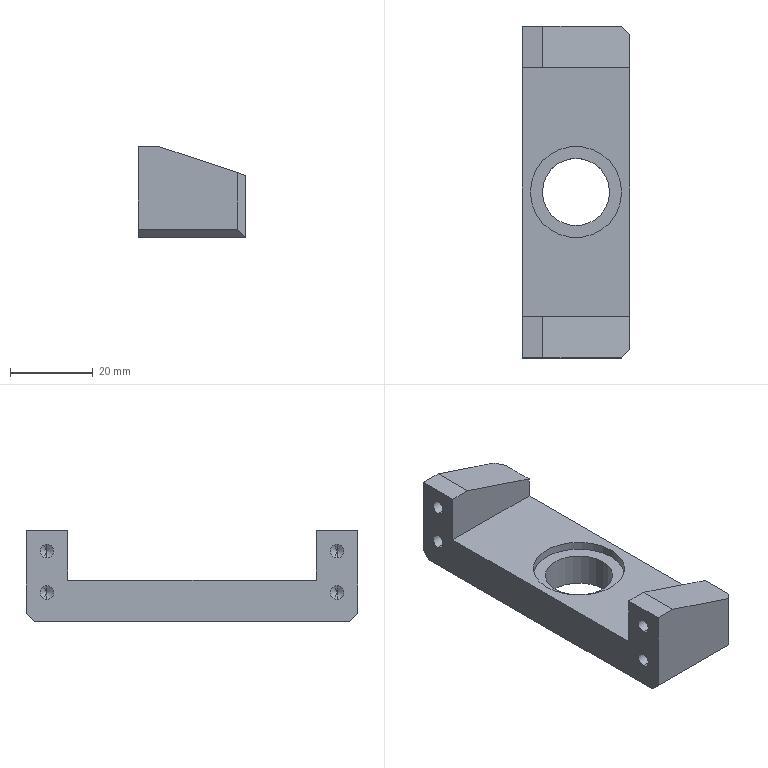Part | SolidWorks | features Chamfer 2, Cut 2, Extrusion 1, HoleWzd 1, ICE 1, MirrorPattern 1 | 1 solid | 37 faces | box 26 x 80 x 22 mm | volume 22644 mm3 | plane 17 | cylinder 12 | cone 8 | commonest cylinder face diameters 3.3 x8 16.2 x2 22 x2
STEP:
#1=CARTESIAN_POINT('',(-2.9,35.,15.35));
#2=VERTEX_POINT('',#1);
#3=CARTESIAN_POINT('',(-2.9,35.,18.65));
#4=VERTEX_POINT('',#3);
#5=CARTESIAN_POINT('',(-2.9,35.,17.));
#6=DIRECTION('',(-1.,0.,0.));
#7=DIRECTION('',(0.,0.,1.));
#8=AXIS2_PLACEMENT_3D('',#5,#6,#7);
#9=CIRCLE('',#8,1.65);
#10=EDGE_CURVE('',#2,#4,#9,.T.);
#11=ORIENTED_EDGE('',*,*,#10,.F.);
#12=CARTESIAN_POINT('',(-13.,35.,15.35));
#13=VERTEX_POINT('',#12);
#14=CARTESIAN_POINT('',(-13.,35.,15.35));
#15=DIRECTION('',(-1.,0.,0.));
#16=VECTOR('',#15,1000.);
#17=LINE('',#14,#16);
#18=EDGE_CURVE('',#2,#13,#17,.T.);
#19=ORIENTED_EDGE('',*,*,#18,.T.);
#20=CARTESIAN_POINT('',(-13.,35.,18.65));
#21=VERTEX_POINT('',#20);
#22=CARTESIAN_POINT('',(-13.,35.,17.));
#23=DIRECTION('',(-1.,0.,0.));
#24=DIRECTION('',(0.,0.,1.));
#25=AXIS2_PLACEMENT_3D('',#22,#23,#24);
#26=CIRCLE('',#25,1.65);
#27=EDGE_CURVE('',#13,#21,#26,.T.);
#28=ORIENTED_EDGE('',*,*,#27,.T.);
#29=CARTESIAN_POINT('',(-13.,35.,18.65));
#30=DIRECTION('',(-1.,0.,0.));
#31=VECTOR('',#30,1000.);
#32=LINE('',#29,#31);
#33=EDGE_CURVE('',#4,#21,#32,.T.);
#34=ORIENTED_EDGE('',*,*,#33,.F.);
#35=EDGE_LOOP('',(#11,#19,#28,#34));
#36=FACE_OUTER_BOUND('',#35,.T.);
#37=CARTESIAN_POINT('',(-13.,35.,17.));
#38=DIRECTION('',(-1.,0.,0.));
#39=DIRECTION('',(0.,0.,1.));
#40=AXIS2_PLACEMENT_3D('',#37,#38,#39);
#41=CYLINDRICAL_SURFACE('',#40,1.65);
#42=ADVANCED_FACE('',(#36),#41,.F.);
#43=CARTESIAN_POINT('',(-1.909,35.,17.));
#44=VERTEX_POINT('',#43);
#45=CARTESIAN_POINT('',(-2.9,35.,18.65));
#46=DIRECTION('',(-0.515,0.,0.8572));
#47=VECTOR('',#46,1000.);
#48=LINE('',#45,#47);
#49=EDGE_CURVE('',#44,#4,#48,.T.);
#50=ORIENTED_EDGE('',*,*,#49,.F.);
#51=CARTESIAN_POINT('',(-2.9,35.,15.35));
#52=DIRECTION('',(-0.515,0.,-0.8572));
#53=VECTOR('',#52,1000.);
#54=LINE('',#51,#53);
#55=EDGE_CURVE('',#44,#2,#54,.T.);
#56=ORIENTED_EDGE('',*,*,#55,.T.);
#57=ORIENTED_EDGE('',*,*,#10,.T.);
#58=EDGE_LOOP('',(#50,#56,#57));
#59=FACE_OUTER_BOUND('',#58,.T.);
#60=CARTESIAN_POINT('',(-2.9,35.,17.));
#61=DIRECTION('',(-1.,0.,0.));
#62=DIRECTION('',(0.,0.,1.));
#63=AXIS2_PLACEMENT_3D('',#60,#61,#62);
#64=CONICAL_SURFACE('',#63,1.65,1.03);
#65=ADVANCED_FACE('',(#59),#64,.F.);
#66=CARTESIAN_POINT('',(-2.9,35.,5.35));
#67=VERTEX_POINT('',#66);
#68=CARTESIAN_POINT('',(-2.9,35.,8.65));
#69=VERTEX_POINT('',#68);
#70=CARTESIAN_POINT('',(-2.9,35.,7.));
#71=DIRECTION('',(-1.,0.,0.));
#72=DIRECTION('',(0.,0.,1.));
#73=AXIS2_PLACEMENT_3D('',#70,#71,#72);
#74=CIRCLE('',#73,1.65);
#75=EDGE_CURVE('',#67,#69,#74,.T.);
#76=ORIENTED_EDGE('',*,*,#75,.F.);
#77=CARTESIAN_POINT('',(-13.,35.,5.35));
#78=VERTEX_POINT('',#77);
#79=CARTESIAN_POINT('',(-13.,35.,5.35));
#80=DIRECTION('',(-1.,0.,0.));
#81=VECTOR('',#80,1000.);
#82=LINE('',#79,#81);
#83=EDGE_CURVE('',#67,#78,#82,.T.);
#84=ORIENTED_EDGE('',*,*,#83,.T.);
#85=CARTESIAN_POINT('',(-13.,35.,8.65));
#86=VERTEX_POINT('',#85);
#87=CARTESIAN_POINT('',(-13.,35.,7.));
#88=DIRECTION('',(-1.,0.,0.));
#89=DIRECTION('',(0.,0.,1.));
#90=AXIS2_PLACEMENT_3D('',#87,#88,#89);
#91=CIRCLE('',#90,1.65);
#92=EDGE_CURVE('',#78,#86,#91,.T.);
#93=ORIENTED_EDGE('',*,*,#92,.T.);
#94=CARTESIAN_POINT('',(-13.,35.,8.65));
#95=DIRECTION('',(-1.,0.,0.));
#96=VECTOR('',#95,1000.);
#97=LINE('',#94,#96);
#98=EDGE_CURVE('',#69,#86,#97,.T.);
#99=ORIENTED_EDGE('',*,*,#98,.F.);
#100=EDGE_LOOP('',(#76,#84,#93,#99));
#101=FACE_OUTER_BOUND('',#100,.T.);
#102=CARTESIAN_POINT('',(-13.,35.,7.));
#103=DIRECTION('',(-1.,0.,0.));
#104=DIRECTION('',(0.,0.,1.));
#105=AXIS2_PLACEMENT_3D('',#102,#103,#104);
#106=CYLINDRICAL_SURFACE('',#105,1.65);
#107=ADVANCED_FACE('',(#101),#106,.F.);
#108=CARTESIAN_POINT('',(-1.909,35.,7.));
#109=VERTEX_POINT('',#108);
#110=CARTESIAN_POINT('',(-2.9,35.,8.65));
#111=DIRECTION('',(-0.515,0.,0.8572));
#112=VECTOR('',#111,1000.);
#113=LINE('',#110,#112);
#114=EDGE_CURVE('',#109,#69,#113,.T.);
#115=ORIENTED_EDGE('',*,*,#114,.F.);
#116=CARTESIAN_POINT('',(-2.9,35.,5.35));
#117=DIRECTION('',(-0.515,0.,-0.8572));
#118=VECTOR('',#117,1000.);
#119=LINE('',#116,#118);
#120=EDGE_CURVE('',#109,#67,#119,.T.);
#121=ORIENTED_EDGE('',*,*,#120,.T.);
#122=ORIENTED_EDGE('',*,*,#75,.T.);
#123=EDGE_LOOP('',(#115,#121,#122));
#124=FACE_OUTER_BOUND('',#123,.T.);
#125=CARTESIAN_POINT('',(-2.9,35.,7.));
#126=DIRECTION('',(-1.,0.,0.));
#127=DIRECTION('',(0.,0.,1.));
#128=AXIS2_PLACEMENT_3D('',#125,#126,#127);
#129=CONICAL_SURFACE('',#128,1.65,1.03);
#130=ADVANCED_FACE('',(#124),#129,.F.);
#131=CARTESIAN_POINT('',(-2.9,-35.,5.35));
#132=VERTEX_POINT('',#131);
#133=CARTESIAN_POINT('',(-2.9,-35.,8.65));
#134=VERTEX_POINT('',#133);
#135=CARTESIAN_POINT('',(-2.9,-35.,7.));
#136=DIRECTION('',(-1.,0.,0.));
#137=DIRECTION('',(0.,0.,1.));
#138=AXIS2_PLACEMENT_3D('',#135,#136,#137);
#139=CIRCLE('',#138,1.65);
#140=EDGE_CURVE('',#132,#134,#139,.T.);
#141=ORIENTED_EDGE('',*,*,#140,.F.);
#142=CARTESIAN_POINT('',(-13.,-35.,5.35));
#143=VERTEX_POINT('',#142);
#144=CARTESIAN_POINT('',(-13.,-35.,5.35));
#145=DIRECTION('',(-1.,0.,0.));
#146=VECTOR('',#145,1000.);
#147=LINE('',#144,#146);
#148=EDGE_CURVE('',#132,#143,#147,.T.);
#149=ORIENTED_EDGE('',*,*,#148,.T.);
#150=CARTESIAN_POINT('',(-13.,-35.,8.65));
#151=VERTEX_POINT('',#150);
#152=CARTESIAN_POINT('',(-13.,-35.,7.));
#153=DIRECTION('',(-1.,0.,0.));
#154=DIRECTION('',(0.,0.,1.));
#155=AXIS2_PLACEMENT_3D('',#152,#153,#154);
#156=CIRCLE('',#155,1.65);
#157=EDGE_CURVE('',#143,#151,#156,.T.);
#158=ORIENTED_EDGE('',*,*,#157,.T.);
#159=CARTESIAN_POINT('',(-13.,-35.,8.65));
#160=DIRECTION('',(-1.,0.,0.));
#161=VECTOR('',#160,1000.);
#162=LINE('',#159,#161);
#163=EDGE_CURVE('',#134,#151,#162,.T.);
#164=ORIENTED_EDGE('',*,*,#163,.F.);
#165=EDGE_LOOP('',(#141,#149,#158,#164));
#166=FACE_OUTER_BOUND('',#165,.T.);
#167=CARTESIAN_POINT('',(-13.,-35.,7.));
#168=DIRECTION('',(-1.,0.,0.));
#169=DIRECTION('',(0.,0.,1.));
#170=AXIS2_PLACEMENT_3D('',#167,#168,#169);
#171=CYLINDRICAL_SURFACE('',#170,1.65);
#172=ADVANCED_FACE('',(#166),#171,.F.);
#173=CARTESIAN_POINT('',(-1.909,-35.,7.));
#174=VERTEX_POINT('',#173);
#175=CARTESIAN_POINT('',(-2.9,-35.,8.65));
#176=DIRECTION('',(-0.515,0.,0.8572));
#177=VECTOR('',#176,1000.);
#178=LINE('',#175,#177);
#179=EDGE_CURVE('',#174,#134,#178,.T.);
#180=ORIENTED_EDGE('',*,*,#179,.F.);
#181=CARTESIAN_POINT('',(-2.9,-35.,5.35));
#182=DIRECTION('',(-0.515,0.,-0.8572));
#183=VECTOR('',#182,1000.);
#184=LINE('',#181,#183);
#185=EDGE_CURVE('',#174,#132,#184,.T.);
#186=ORIENTED_EDGE('',*,*,#185,.T.);
#187=ORIENTED_EDGE('',*,*,#140,.T.);
#188=EDGE_LOOP('',(#180,#186,#187));
#189=FACE_OUTER_BOUND('',#188,.T.);
#190=CARTESIAN_POINT('',(-2.9,-35.,7.));
#191=DIRECTION('',(-1.,0.,0.));
#192=DIRECTION('',(0.,0.,1.));
#193=AXIS2_PLACEMENT_3D('',#190,#191,#192);
#194=CONICAL_SURFACE('',#193,1.65,1.03);
#195=ADVANCED_FACE('',(#189),#194,.F.);
#196=CARTESIAN_POINT('',(-2.9,-35.,15.35));
#197=VERTEX_POINT('',#196);
#198=CARTESIAN_POINT('',(-2.9,-35.,18.65));
#199=VERTEX_POINT('',#198);
#200=CARTESIAN_POINT('',(-2.9,-35.,17.));
#201=DIRECTION('',(-1.,0.,0.));
#202=DIRECTION('',(0.,0.,1.));
#203=AXIS2_PLACEMENT_3D('',#200,#201,#202);
#204=CIRCLE('',#203,1.65);
#205=EDGE_CURVE('',#197,#199,#204,.T.);
#206=ORIENTED_EDGE('',*,*,#205,.F.);
#207=CARTESIAN_POINT('',(-13.,-35.,15.35));
#208=VERTEX_POINT('',#207);
#209=CARTESIAN_POINT('',(-13.,-35.,15.35));
#210=DIRECTION('',(-1.,0.,0.));
#211=VECTOR('',#210,1000.);
#212=LINE('',#209,#211);
#213=EDGE_CURVE('',#197,#208,#212,.T.);
#214=ORIENTED_EDGE('',*,*,#213,.T.);
#215=CARTESIAN_POINT('',(-13.,-35.,18.65));
#216=VERTEX_POINT('',#215);
#217=CARTESIAN_POINT('',(-13.,-35.,17.));
#218=DIRECTION('',(-1.,0.,0.));
#219=DIRECTION('',(0.,0.,1.));
#220=AXIS2_PLACEMENT_3D('',#217,#218,#219);
#221=CIRCLE('',#220,1.65);
#222=EDGE_CURVE('',#208,#216,#221,.T.);
#223=ORIENTED_EDGE('',*,*,#222,.T.);
#224=CARTESIAN_POINT('',(-13.,-35.,18.65));
#225=DIRECTION('',(-1.,0.,0.));
#226=VECTOR('',#225,1000.);
#227=LINE('',#224,#226);
#228=EDGE_CURVE('',#199,#216,#227,.T.);
#229=ORIENTED_EDGE('',*,*,#228,.F.);
#230=EDGE_LOOP('',(#206,#214,#223,#229));
#231=FACE_OUTER_BOUND('',#230,.T.);
#232=CARTESIAN_POINT('',(-13.,-35.,17.));
#233=DIRECTION('',(-1.,0.,0.));
#234=DIRECTION('',(0.,0.,1.));
#235=AXIS2_PLACEMENT_3D('',#232,#233,#234);
#236=CYLINDRICAL_SURFACE('',#235,1.65);
#237=ADVANCED_FACE('',(#231),#236,.F.);
#238=CARTESIAN_POINT('',(-1.909,-35.,17.));
#239=VERTEX_POINT('',#238);
#240=CARTESIAN_POINT('',(-2.9,-35.,18.65));
#241=DIRECTION('',(-0.515,0.,0.8572));
#242=VECTOR('',#241,1000.);
#243=LINE('',#240,#242);
#244=EDGE_CURVE('',#239,#199,#243,.T.);
#245=ORIENTED_EDGE('',*,*,#244,.F.);
#246=CARTESIAN_POINT('',(-2.9,-35.,15.35));
#247=DIRECTION('',(-0.515,0.,-0.8572));
#248=VECTOR('',#247,1000.);
#249=LINE('',#246,#248);
#250=EDGE_CURVE('',#239,#197,#249,.T.);
#251=ORIENTED_EDGE('',*,*,#250,.T.);
#252=ORIENTED_EDGE('',*,*,#205,.T.);
#253=EDGE_LOOP('',(#245,#251,#252));
#254=FACE_OUTER_BOUND('',#253,.T.);
#255=CARTESIAN_POINT('',(-2.9,-35.,17.));
#256=DIRECTION('',(-1.,0.,0.));
#257=DIRECTION('',(0.,0.,1.));
#258=AXIS2_PLACEMENT_3D('',#255,#256,#257);
#259=CONICAL_SURFACE('',#258,1.65,1.03);
#260=ADVANCED_FACE('',(#254),#259,.F.);
#261=CARTESIAN_POINT('',(11.,0.,8.));
#262=VERTEX_POINT('',#261);
#263=CARTESIAN_POINT('',(-11.,0.,8.));
#264=VERTEX_POINT('',#263);
#265=CARTESIAN_POINT('',(0.,0.,8.));
#266=DIRECTION('',(0.,0.,-1.));
#267=DIRECTION('',(-1.,0.,0.));
#268=AXIS2_PLACEMENT_3D('',#265,#266,#267);
#269=CIRCLE('',#268,11.);
#270=EDGE_CURVE('',#262,#264,#269,.T.);
#271=ORIENTED_EDGE('',*,*,#270,.T.);
#272=CARTESIAN_POINT('',(-11.,0.,10.));
#273=VERTEX_POINT('',#272);
#274=CARTESIAN_POINT('',(-11.,0.,8.));
#275=DIRECTION('',(0.,0.,1.));
#276=VECTOR('',#275,1000.);
#277=LINE('',#274,#276);
#278=EDGE_CURVE('',#264,#273,#277,.T.);
#279=ORIENTED_EDGE('',*,*,#278,.T.);
#280=CARTESIAN_POINT('',(11.,0.,10.));
#281=VERTEX_POINT('',#280);
#282=CARTESIAN_POINT('',(0.,0.,10.));
#283=DIRECTION('',(0.,0.,-1.));
#284=DIRECTION('',(-1.,0.,0.));
#285=AXIS2_PLACEMENT_3D('',#282,#283,#284);
#286=CIRCLE('',#285,11.);
#287=EDGE_CURVE('',#281,#273,#286,.T.);
#288=ORIENTED_EDGE('',*,*,#287,.F.);
#289=CARTESIAN_POINT('',(11.,0.,8.));
#290=DIRECTION('',(0.,0.,1.));
#291=VECTOR('',#290,1000.);
#292=LINE('',#289,#291);
#293=EDGE_CURVE('',#262,#281,#292,.T.);
#294=ORIENTED_EDGE('',*,*,#293,.F.);
#295=EDGE_LOOP('',(#271,#279,#288,#294));
#296=FACE_OUTER_BOUND('',#295,.T.);
#297=CARTESIAN_POINT('',(0.,0.,8.));
#298=DIRECTION('',(0.,0.,1.));
#299=DIRECTION('',(1.,0.,0.));
#300=AXIS2_PLACEMENT_3D('',#297,#298,#299);
#301=CYLINDRICAL_SURFACE('',#300,11.);
#302=ADVANCED_FACE('',(#296),#301,.F.);
#303=CARTESIAN_POINT('',(-8.1,0.,0.));
#304=VERTEX_POINT('',#303);
#305=CARTESIAN_POINT('',(8.1,0.,0.));
#306=VERTEX_POINT('',#305);
#307=CARTESIAN_POINT('',(0.,0.,0.));
#308=DIRECTION('',(0.,0.,1.));
#309=DIRECTION('',(1.,0.,0.));
#310=AXIS2_PLACEMENT_3D('',#307,#308,#309);
#311=CIRCLE('',#310,8.1);
#312=EDGE_CURVE('',#304,#306,#311,.T.);
#313=ORIENTED_EDGE('',*,*,#312,.F.);
#314=CARTESIAN_POINT('',(-8.1,0.,8.));
#315=VERTEX_POINT('',#314);
#316=CARTESIAN_POINT('',(-8.1,0.,0.));
#317=DIRECTION('',(0.,0.,1.));
#318=VECTOR('',#317,1000.);
#319=LINE('',#316,#318);
#320=EDGE_CURVE('',#304,#315,#319,.T.);
#321=ORIENTED_EDGE('',*,*,#320,.T.);
#322=CARTESIAN_POINT('',(8.1,0.,8.));
#323=VERTEX_POINT('',#322);
#324=CARTESIAN_POINT('',(0.,0.,8.));
#325=DIRECTION('',(0.,0.,1.));
#326=DIRECTION('',(-1.,0.,0.));
#327=AXIS2_PLACEMENT_3D('',#324,#325,#326);
#328=CIRCLE('',#327,8.1);
#329=EDGE_CURVE('',#315,#323,#328,.T.);
#330=ORIENTED_EDGE('',*,*,#329,.T.);
#331=CARTESIAN_POINT('',(8.1,0.,0.));
#332=DIRECTION('',(0.,0.,1.));
#333=VECTOR('',#332,1000.);
#334=LINE('',#331,#333);
#335=EDGE_CURVE('',#306,#323,#334,.T.);
#336=ORIENTED_EDGE('',*,*,#335,.F.);
#337=EDGE_LOOP('',(#313,#321,#330,#336));
#338=FACE_OUTER_BOUND('',#337,.T.);
#339=CARTESIAN_POINT('',(0.,0.,0.));
#340=DIRECTION('',(0.,0.,1.));
#341=DIRECTION('',(1.,0.,0.));
#342=AXIS2_PLACEMENT_3D('',#339,#340,#341);
#343=CYLINDRICAL_SURFACE('',#342,8.1);
#344=ADVANCED_FACE('',(#338),#343,.F.);
#345=CARTESIAN_POINT('',(-13.,35.,17.));
#346=DIRECTION('',(-1.,0.,0.));
#347=DIRECTION('',(0.,0.,1.));
#348=AXIS2_PLACEMENT_3D('',#345,#346,#347);
#349=CIRCLE('',#348,1.65);
#350=EDGE_CURVE('',#21,#13,#349,.T.);
#351=ORIENTED_EDGE('',*,*,#350,.F.);
#352=ORIENTED_EDGE('',*,*,#27,.F.);
#353=EDGE_LOOP('',(#351,#352));
#354=FACE_BOUND('',#353,.T.);
#355=CARTESIAN_POINT('',(-13.,35.,7.));
#356=DIRECTION('',(-1.,0.,0.));
#357=DIRECTION('',(0.,0.,1.));
#358=AXIS2_PLACEMENT_3D('',#355,#356,#357);
#359=CIRCLE('',#358,1.65);
#360=EDGE_CURVE('',#86,#78,#359,.T.);
#361=ORIENTED_EDGE('',*,*,#360,.F.);
#362=ORIENTED_EDGE('',*,*,#92,.F.);
#363=EDGE_LOOP('',(#361,#362));
#364=FACE_BOUND('',#363,.T.);
#365=CARTESIAN_POINT('',(-13.,-35.,7.));
#366=DIRECTION('',(-1.,0.,0.));
#367=DIRECTION('',(0.,0.,1.));
#368=AXIS2_PLACEMENT_3D('',#365,#366,#367);
#369=CIRCLE('',#368,1.65);
#370=EDGE_CURVE('',#151,#143,#369,.T.);
#371=ORIENTED_EDGE('',*,*,#370,.F.);
#372=ORIENTED_EDGE('',*,*,#157,.F.);
#373=EDGE_LOOP('',(#371,#372));
#374=FACE_BOUND('',#373,.T.);
#375=CARTESIAN_POINT('',(-13.,-35.,17.));
#376=DIRECTION('',(-1.,0.,0.));
#377=DIRECTION('',(0.,0.,1.));
#378=AXIS2_PLACEMENT_3D('',#375,#376,#377);
#379=CIRCLE('',#378,1.65);
#380=EDGE_CURVE('',#216,#208,#379,.T.);
#381=ORIENTED_EDGE('',*,*,#380,.F.);
#382=ORIENTED_EDGE('',*,*,#222,.F.);
#383=EDGE_LOOP('',(#381,#382));
#384=FACE_BOUND('',#383,.T.);
#385=CARTESIAN_POINT('',(-13.,-38.,0.));
#386=VERTEX_POINT('',#385);
#387=CARTESIAN_POINT('',(-13.,38.,0.));
#388=VERTEX_POINT('',#387);
#389=CARTESIAN_POINT('',(-13.,-40.,0.));
#390=DIRECTION('',(0.,1.,0.));
#391=VECTOR('',#390,1000.);
#392=LINE('',#389,#391);
#393=EDGE_CURVE('',#386,#388,#392,.T.);
#394=ORIENTED_EDGE('',*,*,#393,.F.);
#395=CARTESIAN_POINT('',(-13.,-40.,2.));
#396=VERTEX_POINT('',#395);
#397=CARTESIAN_POINT('',(-13.,-44.,6.));
#398=DIRECTION('',(0.,-0.7071,0.7071));
#399=VECTOR('',#398,1000.);
#400=LINE('',#397,#399);
#401=EDGE_CURVE('',#386,#396,#400,.T.);
#402=ORIENTED_EDGE('',*,*,#401,.T.);
#403=CARTESIAN_POINT('',(-13.,-40.,22.));
#404=VERTEX_POINT('',#403);
#405=CARTESIAN_POINT('',(-13.,-40.,10.));
#406=DIRECTION('',(0.,0.,-1.));
#407=VECTOR('',#406,1000.);
#408=LINE('',#405,#407);
#409=EDGE_CURVE('',#404,#396,#408,.T.);
#410=ORIENTED_EDGE('',*,*,#409,.F.);
#411=CARTESIAN_POINT('',(-13.,-30.,22.));
#412=VERTEX_POINT('',#411);
#413=CARTESIAN_POINT('',(-13.,-30.,22.));
#414=DIRECTION('',(0.,-1.,0.));
#415=VECTOR('',#414,1000.);
#416=LINE('',#413,#415);
#417=EDGE_CURVE('',#412,#404,#416,.T.);
#418=ORIENTED_EDGE('',*,*,#417,.F.);
#419=CARTESIAN_POINT('',(-13.,-30.,10.));
#420=VERTEX_POINT('',#419);
#421=CARTESIAN_POINT('',(-13.,-30.,22.));
#422=DIRECTION('',(0.,0.,1.));
#423=VECTOR('',#422,1000.);
#424=LINE('',#421,#423);
#425=EDGE_CURVE('',#420,#412,#424,.T.);
#426=ORIENTED_EDGE('',*,*,#425,.F.);
#427=CARTESIAN_POINT('',(-13.,30.,10.));
#428=VERTEX_POINT('',#427);
#429=CARTESIAN_POINT('',(-13.,-40.,10.));
#430=DIRECTION('',(0.,1.,0.));
#431=VECTOR('',#430,1000.);
#432=LINE('',#429,#431);
#433=EDGE_CURVE('',#420,#428,#432,.T.);
#434=ORIENTED_EDGE('',*,*,#433,.T.);
#435=CARTESIAN_POINT('',(-13.,30.,22.));
#436=VERTEX_POINT('',#435);
#437=CARTESIAN_POINT('',(-13.,30.,22.));
#438=DIRECTION('',(0.,0.,1.));
#439=VECTOR('',#438,1000.);
#440=LINE('',#437,#439);
#441=EDGE_CURVE('',#428,#436,#440,.T.);
#442=ORIENTED_EDGE('',*,*,#441,.T.);
#443=CARTESIAN_POINT('',(-13.,40.,22.));
#444=VERTEX_POINT('',#443);
#445=CARTESIAN_POINT('',(-13.,30.,22.));
#446=DIRECTION('',(0.,1.,0.));
#447=VECTOR('',#446,1000.);
#448=LINE('',#445,#447);
#449=EDGE_CURVE('',#436,#444,#448,.T.);
#450=ORIENTED_EDGE('',*,*,#449,.T.);
#451=CARTESIAN_POINT('',(-13.,40.,2.));
#452=VERTEX_POINT('',#451);
#453=CARTESIAN_POINT('',(-13.,40.,10.));
#454=DIRECTION('',(0.,0.,-1.));
#455=VECTOR('',#454,1000.);
#456=LINE('',#453,#455);
#457=EDGE_CURVE('',#444,#452,#456,.T.);
#458=ORIENTED_EDGE('',*,*,#457,.T.);
#459=CARTESIAN_POINT('',(-13.,4.,-34.));
#460=DIRECTION('',(0.,-0.7071,-0.7071));
#461=VECTOR('',#460,1000.);
#462=LINE('',#459,#461);
#463=EDGE_CURVE('',#452,#388,#462,.T.);
#464=ORIENTED_EDGE('',*,*,#463,.T.);
#465=EDGE_LOOP('',(#394,#402,#410,#418,#426,#434,#442,#450,#458,#464));
#466=FACE_OUTER_BOUND('',#465,.T.);
#467=CARTESIAN_POINT('',(-13.,-40.,10.));
#468=DIRECTION('',(-1.,0.,0.));
#469=DIRECTION('',(0.,0.,1.));
#470=AXIS2_PLACEMENT_3D('',#467,#468,#469);
#471=PLANE('',#470);
#472=ADVANCED_FACE('',(#354,#364,#374,#384,#466),#471,.T.);
#473=ORIENTED_EDGE('',*,*,#409,.T.);
#474=CARTESIAN_POINT('',(11.,-40.,2.));
#475=VERTEX_POINT('',#474);
#476=CARTESIAN_POINT('',(11.,-40.,2.));
#477=DIRECTION('',(1.,0.,0.));
#478=VECTOR('',#477,1000.);
#479=LINE('',#476,#478);
#480=EDGE_CURVE('',#396,#475,#479,.T.);
#481=ORIENTED_EDGE('',*,*,#480,.T.);
#482=CARTESIAN_POINT('',(11.,-40.,15.667));
#483=VERTEX_POINT('',#482);
#484=CARTESIAN_POINT('',(11.,-40.,10.));
#485=DIRECTION('',(0.,0.,1.));
#486=VECTOR('',#485,1000.);
#487=LINE('',#484,#486);
#488=EDGE_CURVE('',#475,#483,#487,.T.);
#489=ORIENTED_EDGE('',*,*,#488,.T.);
#490=CARTESIAN_POINT('',(-8.,-40.,22.));
#491=VERTEX_POINT('',#490);
#492=CARTESIAN_POINT('',(-8.,-40.,22.));
#493=DIRECTION('',(0.9487,0.,-0.3162));
#494=VECTOR('',#493,1000.);
#495=LINE('',#492,#494);
#496=EDGE_CURVE('',#491,#483,#495,.T.);
#497=ORIENTED_EDGE('',*,*,#496,.F.);
#498=CARTESIAN_POINT('',(-13.,-40.,22.));
#499=DIRECTION('',(1.,0.,0.));
#500=VECTOR('',#499,1000.);
#501=LINE('',#498,#500);
#502=EDGE_CURVE('',#404,#491,#501,.T.);
#503=ORIENTED_EDGE('',*,*,#502,.F.);
#504=EDGE_LOOP('',(#473,#481,#489,#497,#503));
#505=FACE_OUTER_BOUND('',#504,.T.);
#506=CARTESIAN_POINT('',(-13.,-40.,10.));
#507=DIRECTION('',(0.,1.,0.));
#508=DIRECTION('',(0.,0.,1.));
#509=AXIS2_PLACEMENT_3D('',#506,#507,#508);
#510=PLANE('',#509);
#511=ADVANCED_FACE('',(#505),#510,.F.);
#512=CARTESIAN_POINT('',(13.,-38.,0.));
#513=VERTEX_POINT('',#512);
#514=CARTESIAN_POINT('',(13.,38.,0.));
#515=VERTEX_POINT('',#514);
#516=CARTESIAN_POINT('',(13.,-40.,0.));
#517=DIRECTION('',(0.,1.,0.));
#518=VECTOR('',#517,1000.);
#519=LINE('',#516,#518);
#520=EDGE_CURVE('',#513,#515,#519,.T.);
#521=ORIENTED_EDGE('',*,*,#520,.T.);
#522=CARTESIAN_POINT('',(13.,38.,15.));
#523=VERTEX_POINT('',#522);
#524=CARTESIAN_POINT('',(13.,38.,15.));
#525=DIRECTION('',(0.,0.,1.));
#526=VECTOR('',#525,1000.);
#527=LINE('',#524,#526);
#528=EDGE_CURVE('',#515,#523,#527,.T.);
#529=ORIENTED_EDGE('',*,*,#528,.T.);
#530=CARTESIAN_POINT('',(13.,30.,15.));
#531=VERTEX_POINT('',#530);
#532=CARTESIAN_POINT('',(13.,30.,15.));
#533=DIRECTION('',(0.,1.,0.));
#534=VECTOR('',#533,1000.);
#535=LINE('',#532,#534);
#536=EDGE_CURVE('',#531,#523,#535,.T.);
#537=ORIENTED_EDGE('',*,*,#536,.F.);
#538=CARTESIAN_POINT('',(13.,30.,10.));
#539=VERTEX_POINT('',#538);
#540=CARTESIAN_POINT('',(13.,30.,10.));
#541=DIRECTION('',(0.,0.,-1.));
#542=VECTOR('',#541,1000.);
#543=LINE('',#540,#542);
#544=EDGE_CURVE('',#531,#539,#543,.T.);
#545=ORIENTED_EDGE('',*,*,#544,.T.);
#546=CARTESIAN_POINT('',(13.,-30.,10.));
#547=VERTEX_POINT('',#546);
#548=CARTESIAN_POINT('',(13.,-40.,10.));
#549=DIRECTION('',(0.,1.,0.));
#550=VECTOR('',#549,1000.);
#551=LINE('',#548,#550);
#552=EDGE_CURVE('',#547,#539,#551,.T.);
#553=ORIENTED_EDGE('',*,*,#552,.F.);
#554=CARTESIAN_POINT('',(13.,-30.,15.));
#555=VERTEX_POINT('',#554);
#556=CARTESIAN_POINT('',(13.,-30.,10.));
#557=DIRECTION('',(0.,0.,-1.));
#558=VECTOR('',#557,1000.);
#559=LINE('',#556,#558);
#560=EDGE_CURVE('',#555,#547,#559,.T.);
#561=ORIENTED_EDGE('',*,*,#560,.F.);
#562=CARTESIAN_POINT('',(13.,-38.,15.));
#563=VERTEX_POINT('',#562);
#564=CARTESIAN_POINT('',(13.,-30.,15.));
#565=DIRECTION('',(0.,-1.,0.));
#566=VECTOR('',#565,1000.);
#567=LINE('',#564,#566);
#568=EDGE_CURVE('',#555,#563,#567,.T.);
#569=ORIENTED_EDGE('',*,*,#568,.T.);
#570=CARTESIAN_POINT('',(13.,-38.,10.));
#571=DIRECTION('',(0.,0.,-1.));
#572=VECTOR('',#571,1000.);
#573=LINE('',#570,#572);
#574=EDGE_CURVE('',#563,#513,#573,.T.);
#575=ORIENTED_EDGE('',*,*,#574,.T.);
#576=EDGE_LOOP('',(#521,#529,#537,#545,#553,#561,#569,#575));
#577=FACE_OUTER_BOUND('',#576,.T.);
#578=CARTESIAN_POINT('',(13.,-40.,10.));
#579=DIRECTION('',(-1.,0.,0.));
#580=DIRECTION('',(0.,0.,1.));
#581=AXIS2_PLACEMENT_3D('',#578,#579,#580);
#582=PLANE('',#581);
#583=ADVANCED_FACE('',(#577),#582,.F.);
#584=CARTESIAN_POINT('',(11.,40.,15.667));
#585=VERTEX_POINT('',#584);
#586=CARTESIAN_POINT('',(11.,40.,2.));
#587=VERTEX_POINT('',#586);
#588=CARTESIAN_POINT('',(11.,40.,0.));
#589=DIRECTION('',(0.,0.,-1.));
#590=VECTOR('',#589,1000.);
#591=LINE('',#588,#590);
#592=EDGE_CURVE('',#585,#587,#591,.T.);
#593=ORIENTED_EDGE('',*,*,#592,.T.);
#594=CARTESIAN_POINT('',(-13.,40.,2.));
#595=DIRECTION('',(-1.,0.,0.));
#596=VECTOR('',#595,1000.);
#597=LINE('',#594,#596);
#598=EDGE_CURVE('',#587,#452,#597,.T.);
#599=ORIENTED_EDGE('',*,*,#598,.T.);
#600=ORIENTED_EDGE('',*,*,#457,.F.);
#601=CARTESIAN_POINT('',(-8.,40.,22.));
#602=VERTEX_POINT('',#601);
#603=CARTESIAN_POINT('',(-13.,40.,22.));
#604=DIRECTION('',(1.,0.,0.));
#605=VECTOR('',#604,1000.);
#606=LINE('',#603,#605);
#607=EDGE_CURVE('',#444,#602,#606,.T.);
#608=ORIENTED_EDGE('',*,*,#607,.T.);
#609=CARTESIAN_POINT('',(-8.,40.,22.));
#610=DIRECTION('',(0.9487,0.,-0.3162));
#611=VECTOR('',#610,1000.);
#612=LINE('',#609,#611);
#613=EDGE_CURVE('',#602,#585,#612,.T.);
#614=ORIENTED_EDGE('',*,*,#613,.T.);
#615=EDGE_LOOP('',(#593,#599,#600,#608,#614));
#616=FACE_OUTER_BOUND('',#615,.T.);
#617=CARTESIAN_POINT('',(-13.,40.,10.));
#618=DIRECTION('',(0.,1.,0.));
#619=DIRECTION('',(0.,0.,1.));
#620=AXIS2_PLACEMENT_3D('',#617,#618,#619);
#621=PLANE('',#620);
#622=ADVANCED_FACE('',(#616),#621,.T.);
#623=ORIENTED_EDGE('',*,*,#287,.T.);
#624=CARTESIAN_POINT('',(0.,0.,10.));
#625=DIRECTION('',(0.,0.,-1.));
#626=DIRECTION('',(-1.,0.,0.));
#627=AXIS2_PLACEMENT_3D('',#624,#625,#626);
#628=CIRCLE('',#627,11.);
#629=EDGE_CURVE('',#273,#281,#628,.T.);
#630=ORIENTED_EDGE('',*,*,#629,.T.);
#631=EDGE_LOOP('',(#623,#630));
#632=FACE_BOUND('',#631,.T.);
#633=ORIENTED_EDGE('',*,*,#433,.F.);
#634=CARTESIAN_POINT('',(-13.,-30.,10.));
#635=DIRECTION('',(-1.,0.,0.));
#636=VECTOR('',#635,1000.);
#637=LINE('',#634,#636);
#638=EDGE_CURVE('',#547,#420,#637,.T.);
#639=ORIENTED_EDGE('',*,*,#638,.F.);
#640=ORIENTED_EDGE('',*,*,#552,.T.);
#641=CARTESIAN_POINT('',(-13.,30.,10.));
#642=DIRECTION('',(-1.,0.,0.));
#643=VECTOR('',#642,1000.);
#644=LINE('',#641,#643);
#645=EDGE_CURVE('',#539,#428,#644,.T.);
#646=ORIENTED_EDGE('',*,*,#645,.T.);
#647=EDGE_LOOP('',(#633,#639,#640,#646));
#648=FACE_OUTER_BOUND('',#647,.T.);
#649=CARTESIAN_POINT('',(0.,0.,10.));
#650=DIRECTION('',(0.,0.,-1.));
#651=DIRECTION('',(-1.,0.,0.));
#652=AXIS2_PLACEMENT_3D('',#649,#650,#651);
#653=PLANE('',#652);
#654=ADVANCED_FACE('',(#632,#648),#653,.F.);
#655=CARTESIAN_POINT('',(0.,0.,0.));
#656=DIRECTION('',(0.,0.,1.));
#657=DIRECTION('',(1.,0.,0.));
#658=AXIS2_PLACEMENT_3D('',#655,#656,#657);
#659=CIRCLE('',#658,8.1);
#660=EDGE_CURVE('',#306,#304,#659,.T.);
#661=ORIENTED_EDGE('',*,*,#660,.T.);
#662=ORIENTED_EDGE('',*,*,#312,.T.);
#663=EDGE_LOOP('',(#661,#662));
#664=FACE_BOUND('',#663,.T.);
#665=ORIENTED_EDGE('',*,*,#520,.F.);
#666=CARTESIAN_POINT('',(-13.,-38.,0.));
#667=DIRECTION('',(-1.,0.,0.));
#668=VECTOR('',#667,1000.);
#669=LINE('',#666,#668);
#670=EDGE_CURVE('',#513,#386,#669,.T.);
#671=ORIENTED_EDGE('',*,*,#670,.T.);
#672=ORIENTED_EDGE('',*,*,#393,.T.);
#673=CARTESIAN_POINT('',(0.,38.,0.));
#674=DIRECTION('',(1.,0.,0.));
#675=VECTOR('',#674,1000.);
#676=LINE('',#673,#675);
#677=EDGE_CURVE('',#388,#515,#676,.T.);
#678=ORIENTED_EDGE('',*,*,#677,.T.);
#679=EDGE_LOOP('',(#665,#671,#672,#678));
#680=FACE_OUTER_BOUND('',#679,.T.);
#681=CARTESIAN_POINT('',(0.,0.,0.));
#682=DIRECTION('',(0.,0.,-1.));
#683=DIRECTION('',(-1.,0.,0.));
#684=AXIS2_PLACEMENT_3D('',#681,#682,#683);
#685=PLANE('',#684);
#686=ADVANCED_FACE('',(#664,#680),#685,.T.);
#687=ORIENTED_EDGE('',*,*,#320,.F.);
#688=ORIENTED_EDGE('',*,*,#660,.F.);
#689=ORIENTED_EDGE('',*,*,#335,.T.);
#690=CARTESIAN_POINT('',(0.,0.,8.));
#691=DIRECTION('',(0.,0.,1.));
#692=DIRECTION('',(-1.,0.,0.));
#693=AXIS2_PLACEMENT_3D('',#690,#691,#692);
#694=CIRCLE('',#693,8.1);
#695=EDGE_CURVE('',#323,#315,#694,.T.);
#696=ORIENTED_EDGE('',*,*,#695,.T.);
#697=EDGE_LOOP('',(#687,#688,#689,#696));
#698=FACE_OUTER_BOUND('',#697,.T.);
#699=CARTESIAN_POINT('',(0.,0.,0.));
#700=DIRECTION('',(0.,0.,1.));
#701=DIRECTION('',(1.,0.,0.));
#702=AXIS2_PLACEMENT_3D('',#699,#700,#701);
#703=CYLINDRICAL_SURFACE('',#702,8.1);
#704=ADVANCED_FACE('',(#698),#703,.F.);
#705=ORIENTED_EDGE('',*,*,#536,.T.);
#706=CARTESIAN_POINT('',(5.737,45.263,17.421));
#707=DIRECTION('',(-0.6882,0.6882,0.2294));
#708=VECTOR('',#707,1000.);
#709=LINE('',#706,#708);
#710=EDGE_CURVE('',#523,#585,#709,.T.);
#711=ORIENTED_EDGE('',*,*,#710,.T.);
#712=ORIENTED_EDGE('',*,*,#613,.F.);
#713=CARTESIAN_POINT('',(-8.,30.,22.));
#714=VERTEX_POINT('',#713);
#715=CARTESIAN_POINT('',(-8.,30.,22.));
#716=DIRECTION('',(0.,1.,0.));
#717=VECTOR('',#716,1000.);
#718=LINE('',#715,#717);
#719=EDGE_CURVE('',#714,#602,#718,.T.);
#720=ORIENTED_EDGE('',*,*,#719,.F.);
#721=CARTESIAN_POINT('',(-8.,30.,22.));
#722=DIRECTION('',(0.9487,0.,-0.3162));
#723=VECTOR('',#722,1000.);
#724=LINE('',#721,#723);
#725=EDGE_CURVE('',#714,#531,#724,.T.);
#726=ORIENTED_EDGE('',*,*,#725,.T.);
#727=EDGE_LOOP('',(#705,#711,#712,#720,#726));
#728=FACE_OUTER_BOUND('',#727,.T.);
#729=CARTESIAN_POINT('',(-8.,30.,22.));
#730=DIRECTION('',(0.3162,0.,0.9487));
#731=DIRECTION('',(0.9487,0.,-0.3162));
#732=AXIS2_PLACEMENT_3D('',#729,#730,#731);
#733=PLANE('',#732);
#734=ADVANCED_FACE('',(#728),#733,.T.);
#735=ORIENTED_EDGE('',*,*,#607,.F.);
#736=ORIENTED_EDGE('',*,*,#449,.F.);
#737=CARTESIAN_POINT('',(-13.,30.,22.));
#738=DIRECTION('',(1.,0.,0.));
#739=VECTOR('',#738,1000.);
#740=LINE('',#737,#739);
#741=EDGE_CURVE('',#436,#714,#740,.T.);
#742=ORIENTED_EDGE('',*,*,#741,.T.);
#743=ORIENTED_EDGE('',*,*,#719,.T.);
#744=EDGE_LOOP('',(#735,#736,#742,#743));
#745=FACE_OUTER_BOUND('',#744,.T.);
#746=CARTESIAN_POINT('',(-13.,30.,22.));
#747=DIRECTION('',(0.,0.,1.));
#748=DIRECTION('',(1.,0.,0.));
#749=AXIS2_PLACEMENT_3D('',#746,#747,#748);
#750=PLANE('',#749);
#751=ADVANCED_FACE('',(#745),#750,.T.);
#752=ORIENTED_EDGE('',*,*,#645,.F.);
#753=ORIENTED_EDGE('',*,*,#544,.F.);
#754=ORIENTED_EDGE('',*,*,#725,.F.);
#755=ORIENTED_EDGE('',*,*,#741,.F.);
#756=ORIENTED_EDGE('',*,*,#441,.F.);
#757=EDGE_LOOP('',(#752,#753,#754,#755,#756));
#758=FACE_OUTER_BOUND('',#757,.T.);
#759=CARTESIAN_POINT('',(0.,30.,0.));
#760=DIRECTION('',(0.,-1.,0.));
#761=DIRECTION('',(0.,0.,-1.));
#762=AXIS2_PLACEMENT_3D('',#759,#760,#761);
#763=PLANE('',#762);
#764=ADVANCED_FACE('',(#758),#763,.T.);
#765=ORIENTED_EDGE('',*,*,#502,.T.);
#766=CARTESIAN_POINT('',(-8.,-30.,22.));
#767=VERTEX_POINT('',#766);
#768=CARTESIAN_POINT('',(-8.,-30.,22.));
#769=DIRECTION('',(0.,-1.,0.));
#770=VECTOR('',#769,1000.);
#771=LINE('',#768,#770);
#772=EDGE_CURVE('',#767,#491,#771,.T.);
#773=ORIENTED_EDGE('',*,*,#772,.F.);
#774=CARTESIAN_POINT('',(-13.,-30.,22.));
#775=DIRECTION('',(1.,0.,0.));
#776=VECTOR('',#775,1000.);
#777=LINE('',#774,#776);
#778=EDGE_CURVE('',#412,#767,#777,.T.);
#779=ORIENTED_EDGE('',*,*,#778,.F.);
#780=ORIENTED_EDGE('',*,*,#417,.T.);
#781=EDGE_LOOP('',(#765,#773,#779,#780));
#782=FACE_OUTER_BOUND('',#781,.T.);
#783=CARTESIAN_POINT('',(-13.,-30.,22.));
#784=DIRECTION('',(0.,0.,-1.));
#785=DIRECTION('',(-1.,0.,0.));
#786=AXIS2_PLACEMENT_3D('',#783,#784,#785);
#787=PLANE('',#786);
#788=ADVANCED_FACE('',(#782),#787,.F.);
#789=ORIENTED_EDGE('',*,*,#496,.T.);
#790=CARTESIAN_POINT('',(13.789,-37.211,14.737));
#791=DIRECTION('',(0.6882,0.6882,-0.2294));
#792=VECTOR('',#791,1000.);
#793=LINE('',#790,#792);
#794=EDGE_CURVE('',#483,#563,#793,.T.);
#795=ORIENTED_EDGE('',*,*,#794,.T.);
#796=ORIENTED_EDGE('',*,*,#568,.F.);
#797=CARTESIAN_POINT('',(-8.,-30.,22.));
#798=DIRECTION('',(0.9487,0.,-0.3162));
#799=VECTOR('',#798,1000.);
#800=LINE('',#797,#799);
#801=EDGE_CURVE('',#767,#555,#800,.T.);
#802=ORIENTED_EDGE('',*,*,#801,.F.);
#803=ORIENTED_EDGE('',*,*,#772,.T.);
#804=EDGE_LOOP('',(#789,#795,#796,#802,#803));
#805=FACE_OUTER_BOUND('',#804,.T.);
#806=CARTESIAN_POINT('',(-8.,-30.,22.));
#807=DIRECTION('',(-0.3162,0.,-0.9487));
#808=DIRECTION('',(-0.9487,0.,0.3162));
#809=AXIS2_PLACEMENT_3D('',#806,#807,#808);
#810=PLANE('',#809);
#811=ADVANCED_FACE('',(#805),#810,.F.);
#812=ORIENTED_EDGE('',*,*,#638,.T.);
#813=ORIENTED_EDGE('',*,*,#425,.T.);
#814=ORIENTED_EDGE('',*,*,#778,.T.);
#815=ORIENTED_EDGE('',*,*,#801,.T.);
#816=ORIENTED_EDGE('',*,*,#560,.T.);
#817=EDGE_LOOP('',(#812,#813,#814,#815,#816));
#818=FACE_OUTER_BOUND('',#817,.T.);
#819=CARTESIAN_POINT('',(0.,-30.,0.));
#820=DIRECTION('',(0.,1.,0.));
#821=DIRECTION('',(0.,0.,-1.));
#822=AXIS2_PLACEMENT_3D('',#819,#820,#821);
#823=PLANE('',#822);
#824=ADVANCED_FACE('',(#818),#823,.T.);
#825=ORIENTED_EDGE('',*,*,#528,.F.);
#826=CARTESIAN_POINT('',(8.333,42.667,4.667));
#827=DIRECTION('',(-0.5774,0.5774,0.5774));
#828=VECTOR('',#827,1000.);
#829=LINE('',#826,#828);
#830=EDGE_CURVE('',#515,#587,#829,.T.);
#831=ORIENTED_EDGE('',*,*,#830,.T.);
#832=ORIENTED_EDGE('',*,*,#592,.F.);
#833=ORIENTED_EDGE('',*,*,#710,.F.);
#834=EDGE_LOOP('',(#825,#831,#832,#833));
#835=FACE_OUTER_BOUND('',#834,.T.);
#836=CARTESIAN_POINT('',(11.,40.,10.));
#837=DIRECTION('',(0.7071,0.7071,0.));
#838=DIRECTION('',(0.,0.,1.));
#839=AXIS2_PLACEMENT_3D('',#836,#837,#838);
#840=PLANE('',#839);
#841=ADVANCED_FACE('',(#835),#840,.T.);
#842=ORIENTED_EDGE('',*,*,#488,.F.);
#843=CARTESIAN_POINT('',(9.667,-41.333,3.333));
#844=DIRECTION('',(0.5774,0.5774,-0.5774));
#845=VECTOR('',#844,1000.);
#846=LINE('',#843,#845);
#847=EDGE_CURVE('',#475,#513,#846,.T.);
#848=ORIENTED_EDGE('',*,*,#847,.T.);
#849=ORIENTED_EDGE('',*,*,#574,.F.);
#850=ORIENTED_EDGE('',*,*,#794,.F.);
#851=EDGE_LOOP('',(#842,#848,#849,#850));
#852=FACE_OUTER_BOUND('',#851,.T.);
#853=CARTESIAN_POINT('',(13.,-38.,10.));
#854=DIRECTION('',(-0.7071,0.7071,0.));
#855=DIRECTION('',(0.,0.,-1.));
#856=AXIS2_PLACEMENT_3D('',#853,#854,#855);
#857=PLANE('',#856);
#858=ADVANCED_FACE('',(#852),#857,.F.);
#859=ORIENTED_EDGE('',*,*,#401,.F.);
#860=ORIENTED_EDGE('',*,*,#670,.F.);
#861=ORIENTED_EDGE('',*,*,#847,.F.);
#862=ORIENTED_EDGE('',*,*,#480,.F.);
#863=EDGE_LOOP('',(#859,#860,#861,#862));
#864=FACE_OUTER_BOUND('',#863,.T.);
#865=CARTESIAN_POINT('',(-13.,-40.,2.));
#866=DIRECTION('',(0.,-0.7071,-0.7071));
#867=DIRECTION('',(-1.,0.,0.));
#868=AXIS2_PLACEMENT_3D('',#865,#866,#867);
#869=PLANE('',#868);
#870=ADVANCED_FACE('',(#864),#869,.T.);
#871=ORIENTED_EDGE('',*,*,#463,.F.);
#872=ORIENTED_EDGE('',*,*,#598,.F.);
#873=ORIENTED_EDGE('',*,*,#830,.F.);
#874=ORIENTED_EDGE('',*,*,#677,.F.);
#875=EDGE_LOOP('',(#871,#872,#873,#874));
#876=FACE_OUTER_BOUND('',#875,.T.);
#877=CARTESIAN_POINT('',(0.,38.,0.));
#878=DIRECTION('',(0.,-0.7071,0.7071));
#879=DIRECTION('',(1.,0.,0.));
#880=AXIS2_PLACEMENT_3D('',#877,#878,#879);
#881=PLANE('',#880);
#882=ADVANCED_FACE('',(#876),#881,.F.);
#883=ORIENTED_EDGE('',*,*,#270,.F.);
#884=CARTESIAN_POINT('',(0.,0.,8.));
#885=DIRECTION('',(0.,0.,-1.));
#886=DIRECTION('',(-1.,0.,0.));
#887=AXIS2_PLACEMENT_3D('',#884,#885,#886);
#888=CIRCLE('',#887,11.);
#889=EDGE_CURVE('',#264,#262,#888,.T.);
#890=ORIENTED_EDGE('',*,*,#889,.F.);
#891=EDGE_LOOP('',(#883,#890));
#892=FACE_OUTER_BOUND('',#891,.T.);
#893=ORIENTED_EDGE('',*,*,#695,.F.);
#894=ORIENTED_EDGE('',*,*,#329,.F.);
#895=EDGE_LOOP('',(#893,#894));
#896=FACE_BOUND('',#895,.T.);
#897=CARTESIAN_POINT('',(0.,0.,8.));
#898=DIRECTION('',(0.,0.,-1.));
#899=DIRECTION('',(-1.,0.,0.));
#900=AXIS2_PLACEMENT_3D('',#897,#898,#899);
#901=PLANE('',#900);
#902=ADVANCED_FACE('',(#892,#896),#901,.F.);
#903=ORIENTED_EDGE('',*,*,#278,.F.);
#904=ORIENTED_EDGE('',*,*,#889,.T.);
#905=ORIENTED_EDGE('',*,*,#293,.T.);
#906=ORIENTED_EDGE('',*,*,#629,.F.);
#907=EDGE_LOOP('',(#903,#904,#905,#906));
#908=FACE_OUTER_BOUND('',#907,.T.);
#909=CARTESIAN_POINT('',(0.,0.,8.));
#910=DIRECTION('',(0.,0.,1.));
#911=DIRECTION('',(1.,0.,0.));
#912=AXIS2_PLACEMENT_3D('',#909,#910,#911);
#913=CYLINDRICAL_SURFACE('',#912,11.);
#914=ADVANCED_FACE('',(#908),#913,.F.);
#915=ORIENTED_EDGE('',*,*,#250,.F.);
#916=ORIENTED_EDGE('',*,*,#244,.T.);
#917=CARTESIAN_POINT('',(-2.9,-35.,17.));
#918=DIRECTION('',(-1.,0.,0.));
#919=DIRECTION('',(0.,0.,1.));
#920=AXIS2_PLACEMENT_3D('',#917,#918,#919);
#921=CIRCLE('',#920,1.65);
#922=EDGE_CURVE('',#199,#197,#921,.T.);
#923=ORIENTED_EDGE('',*,*,#922,.T.);
#924=EDGE_LOOP('',(#915,#916,#923));
#925=FACE_OUTER_BOUND('',#924,.T.);
#926=CARTESIAN_POINT('',(-2.9,-35.,17.));
#927=DIRECTION('',(-1.,0.,0.));
#928=DIRECTION('',(0.,0.,1.));
#929=AXIS2_PLACEMENT_3D('',#926,#927,#928);
#930=CONICAL_SURFACE('',#929,1.65,1.03);
#931=ADVANCED_FACE('',(#925),#930,.F.);
#932=ORIENTED_EDGE('',*,*,#213,.F.);
#933=ORIENTED_EDGE('',*,*,#922,.F.);
#934=ORIENTED_EDGE('',*,*,#228,.T.);
#935=ORIENTED_EDGE('',*,*,#380,.T.);
#936=EDGE_LOOP('',(#932,#933,#934,#935));
#937=FACE_OUTER_BOUND('',#936,.T.);
#938=CARTESIAN_POINT('',(-13.,-35.,17.));
#939=DIRECTION('',(-1.,0.,0.));
#940=DIRECTION('',(0.,0.,1.));
#941=AXIS2_PLACEMENT_3D('',#938,#939,#940);
#942=CYLINDRICAL_SURFACE('',#941,1.65);
#943=ADVANCED_FACE('',(#937),#942,.F.);
#944=ORIENTED_EDGE('',*,*,#185,.F.);
#945=ORIENTED_EDGE('',*,*,#179,.T.);
#946=CARTESIAN_POINT('',(-2.9,-35.,7.));
#947=DIRECTION('',(-1.,0.,0.));
#948=DIRECTION('',(0.,0.,1.));
#949=AXIS2_PLACEMENT_3D('',#946,#947,#948);
#950=CIRCLE('',#949,1.65);
#951=EDGE_CURVE('',#134,#132,#950,.T.);
#952=ORIENTED_EDGE('',*,*,#951,.T.);
#953=EDGE_LOOP('',(#944,#945,#952));
#954=FACE_OUTER_BOUND('',#953,.T.);
#955=CARTESIAN_POINT('',(-2.9,-35.,7.));
#956=DIRECTION('',(-1.,0.,0.));
#957=DIRECTION('',(0.,0.,1.));
#958=AXIS2_PLACEMENT_3D('',#955,#956,#957);
#959=CONICAL_SURFACE('',#958,1.65,1.03);
#960=ADVANCED_FACE('',(#954),#959,.F.);
#961=ORIENTED_EDGE('',*,*,#148,.F.);
#962=ORIENTED_EDGE('',*,*,#951,.F.);
#963=ORIENTED_EDGE('',*,*,#163,.T.);
#964=ORIENTED_EDGE('',*,*,#370,.T.);
#965=EDGE_LOOP('',(#961,#962,#963,#964));
#966=FACE_OUTER_BOUND('',#965,.T.);
#967=CARTESIAN_POINT('',(-13.,-35.,7.));
#968=DIRECTION('',(-1.,0.,0.));
#969=DIRECTION('',(0.,0.,1.));
#970=AXIS2_PLACEMENT_3D('',#967,#968,#969);
#971=CYLINDRICAL_SURFACE('',#970,1.65);
#972=ADVANCED_FACE('',(#966),#971,.F.);
#973=ORIENTED_EDGE('',*,*,#120,.F.);
#974=ORIENTED_EDGE('',*,*,#114,.T.);
#975=CARTESIAN_POINT('',(-2.9,35.,7.));
#976=DIRECTION('',(-1.,0.,0.));
#977=DIRECTION('',(0.,0.,1.));
#978=AXIS2_PLACEMENT_3D('',#975,#976,#977);
#979=CIRCLE('',#978,1.65);
#980=EDGE_CURVE('',#69,#67,#979,.T.);
#981=ORIENTED_EDGE('',*,*,#980,.T.);
#982=EDGE_LOOP('',(#973,#974,#981));
#983=FACE_OUTER_BOUND('',#982,.T.);
#984=CARTESIAN_POINT('',(-2.9,35.,7.));
#985=DIRECTION('',(-1.,0.,0.));
#986=DIRECTION('',(0.,0.,1.));
#987=AXIS2_PLACEMENT_3D('',#984,#985,#986);
#988=CONICAL_SURFACE('',#987,1.65,1.03);
#989=ADVANCED_FACE('',(#983),#988,.F.);
#990=ORIENTED_EDGE('',*,*,#83,.F.);
#991=ORIENTED_EDGE('',*,*,#980,.F.);
#992=ORIENTED_EDGE('',*,*,#98,.T.);
#993=ORIENTED_EDGE('',*,*,#360,.T.);
#994=EDGE_LOOP('',(#990,#991,#992,#993));
#995=FACE_OUTER_BOUND('',#994,.T.);
#996=CARTESIAN_POINT('',(-13.,35.,7.));
#997=DIRECTION('',(-1.,0.,0.));
#998=DIRECTION('',(0.,0.,1.));
#999=AXIS2_PLACEMENT_3D('',#996,#997,#998);
#1000=CYLINDRICAL_SURFACE('',#999,1.65);
#1001=ADVANCED_FACE('',(#995),#1000,.F.);
#1002=ORIENTED_EDGE('',*,*,#55,.F.);
#1003=ORIENTED_EDGE('',*,*,#49,.T.);
#1004=CARTESIAN_POINT('',(-2.9,35.,17.));
#1005=DIRECTION('',(-1.,0.,0.));
#1006=DIRECTION('',(0.,0.,1.));
#1007=AXIS2_PLACEMENT_3D('',#1004,#1005,#1006);
#1008=CIRCLE('',#1007,1.65);
#1009=EDGE_CURVE('',#4,#2,#1008,.T.);
#1010=ORIENTED_EDGE('',*,*,#1009,.T.);
#1011=EDGE_LOOP('',(#1002,#1003,#1010));
#1012=FACE_OUTER_BOUND('',#1011,.T.);
#1013=CARTESIAN_POINT('',(-2.9,35.,17.));
#1014=DIRECTION('',(-1.,0.,0.));
#1015=DIRECTION('',(0.,0.,1.));
#1016=AXIS2_PLACEMENT_3D('',#1013,#1014,#1015);
#1017=CONICAL_SURFACE('',#1016,1.65,1.03);
#1018=ADVANCED_FACE('',(#1012),#1017,.F.);
#1019=ORIENTED_EDGE('',*,*,#18,.F.);
#1020=ORIENTED_EDGE('',*,*,#1009,.F.);
#1021=ORIENTED_EDGE('',*,*,#33,.T.);
#1022=ORIENTED_EDGE('',*,*,#350,.T.);
#1023=EDGE_LOOP('',(#1019,#1020,#1021,#1022));
#1024=FACE_OUTER_BOUND('',#1023,.T.);
#1025=CARTESIAN_POINT('',(-13.,35.,17.));
#1026=DIRECTION('',(-1.,0.,0.));
#1027=DIRECTION('',(0.,0.,1.));
#1028=AXIS2_PLACEMENT_3D('',#1025,#1026,#1027);
#1029=CYLINDRICAL_SURFACE('',#1028,1.65);
#1030=ADVANCED_FACE('',(#1024),#1029,.F.);
#1031=CLOSED_SHELL('',(#42,#65,#107,#130,#172,#195,#237,#260,#302,#344,#472,#511,#583,#622,#654,#686,#704,#734,#751,#764,#788,#811,#824,#841,#858,#870,#882,#902,#914,#931,#943,#960,#972,#989,#1001,#1018,#1030));
#1032=MANIFOLD_SOLID_BREP('',#1031);
#1033=CARTESIAN_POINT('',(0.,0.,0.));
#1034=DIRECTION('',(0.,0.,1.));
#1035=DIRECTION('',(1.,0.,0.));
#1036=AXIS2_PLACEMENT_3D('',#1033,#1034,#1035);
#1037=(LENGTH_UNIT()NAMED_UNIT(*)SI_UNIT(.MILLI.,.METRE.));
#1038=UNCERTAINTY_MEASURE_WITH_UNIT(LENGTH_MEASURE(0.00001),#1037,'','');
#1039=(NAMED_UNIT(*)PLANE_ANGLE_UNIT()SI_UNIT($,.RADIAN.));
#1040=(NAMED_UNIT(*)SI_UNIT($,.STERADIAN.)SOLID_ANGLE_UNIT());
#1041=(GEOMETRIC_REPRESENTATION_CONTEXT(3)GLOBAL_UNCERTAINTY_ASSIGNED_CONTEXT((#1038))GLOBAL_UNIT_ASSIGNED_CONTEXT((#1037,#1039,#1040))REPRESENTATION_CONTEXT('',''));
#1042=ADVANCED_BREP_SHAPE_REPRESENTATION('',(#1032,#1036),#1041);